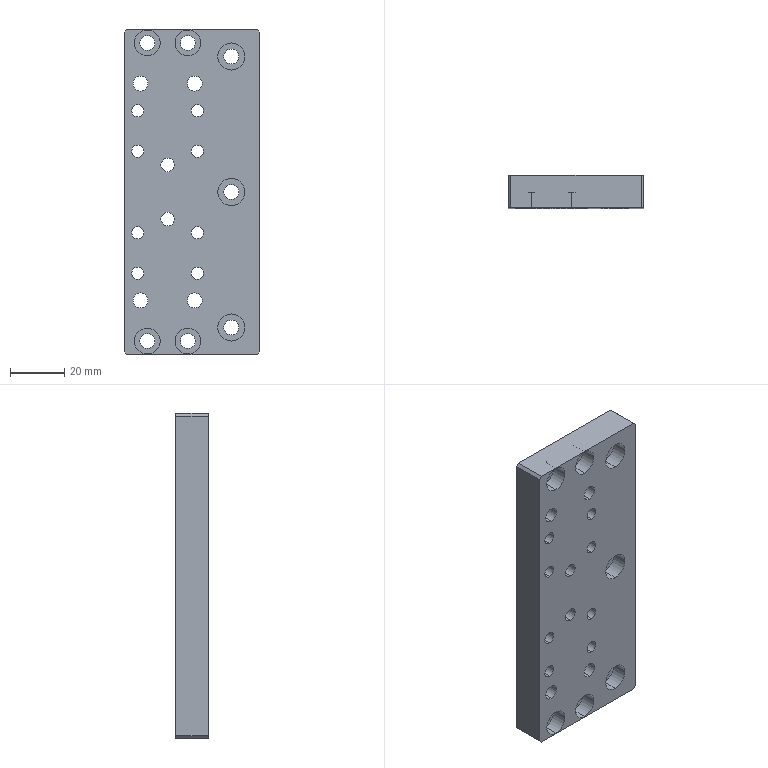Part | SolidWorks | features HoleWzd 5, Chamfer 1, Extrusion 1 | 1 solid | 109 faces | box 50 x 12 x 120 mm | volume 62317 mm3 | cylinder 80 | plane 29 | commonest cylinder face diameters 5.5 x22 4.5 x16 8 x16 10 x14 9.5 x8 5 x4